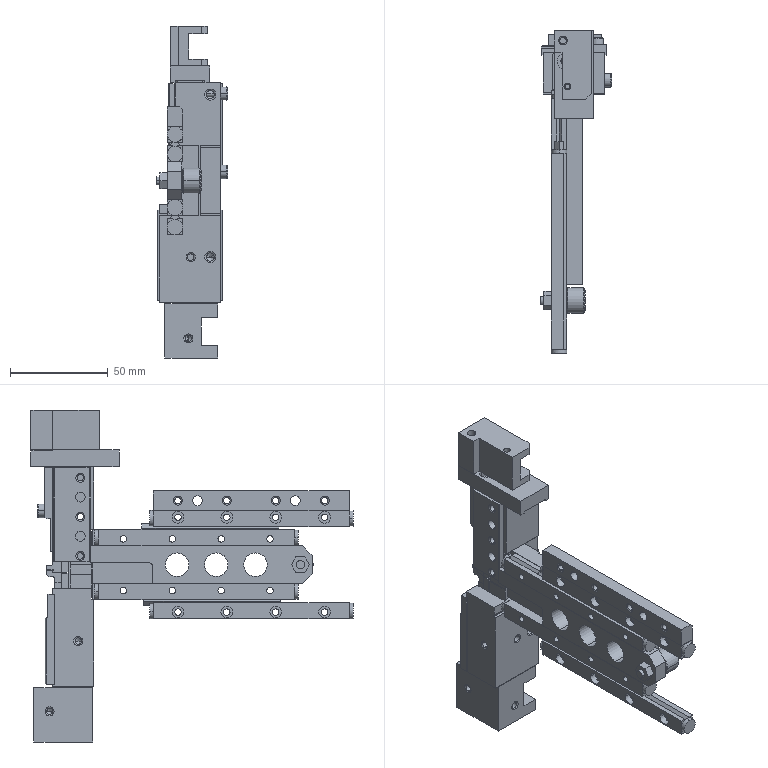Part | NX | 24 solids | 887 faces | box 36.3 x 164.6 x 169.65 mm | volume 170798 mm3 | plane 461 | cylinder 300 | cone 126 | commonest cylinder face diameters 3.3 x74 5 x40 6 x40 8 x36 4.5 x17 3 x14